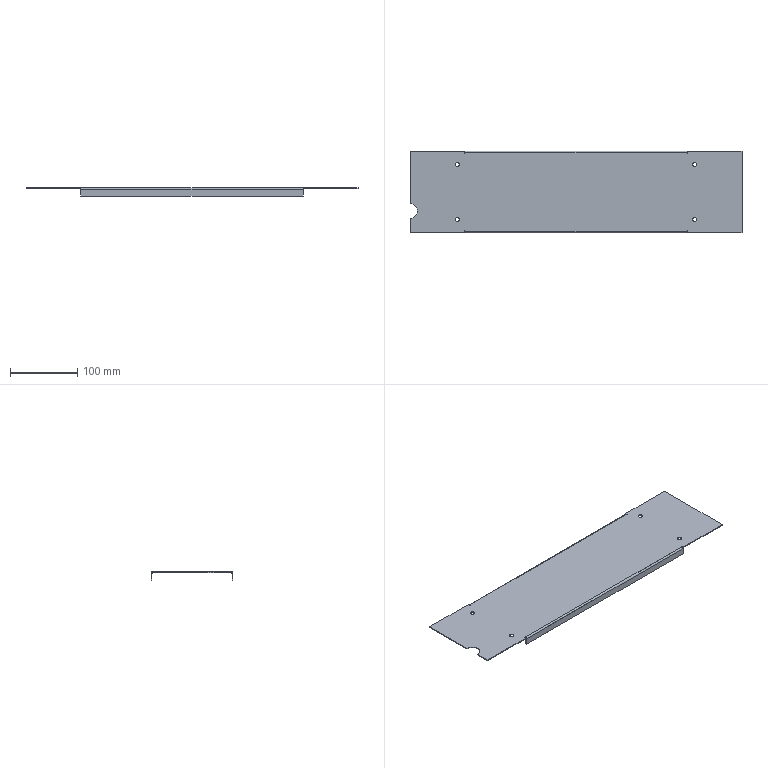Part | SolidWorks | features Cut 2, EdgeFlange 2, FlatPattern 1, SMBaseFlange 1, SheetMetal 1 | 1 solid | 49 faces | box 495 x 122 x 12 mm | volume 80038 mm3 | plane 35 | cylinder 14 | commonest cylinder face diameters 6.5 x8 2.4 x2 4.8 x2 22 x2
STEP:
#1=CARTESIAN_POINT('',(0.,43.5,-1.2));
#2=VERTEX_POINT('',#1);
#3=CARTESIAN_POINT('',(11.,32.5,-1.2));
#4=VERTEX_POINT('',#3);
#5=CARTESIAN_POINT('',(0.,32.5,-1.2));
#6=DIRECTION('',(0.,0.,-1.));
#7=DIRECTION('',(-1.,0.,0.));
#8=AXIS2_PLACEMENT_3D('',#5,#6,#7);
#9=CIRCLE('',#8,11.);
#10=EDGE_CURVE('',#2,#4,#9,.T.);
#11=ORIENTED_EDGE('',*,*,#10,.T.);
#12=CARTESIAN_POINT('',(11.,32.5,0.));
#13=VERTEX_POINT('',#12);
#14=CARTESIAN_POINT('',(11.,32.5,-2.));
#15=DIRECTION('',(0.,0.,1.));
#16=VECTOR('',#15,1000.);
#17=LINE('',#14,#16);
#18=EDGE_CURVE('',#4,#13,#17,.T.);
#19=ORIENTED_EDGE('',*,*,#18,.T.);
#20=CARTESIAN_POINT('',(0.,43.5,0.));
#21=VERTEX_POINT('',#20);
#22=CARTESIAN_POINT('',(0.,32.5,0.));
#23=DIRECTION('',(0.,0.,1.));
#24=DIRECTION('',(1.,0.,0.));
#25=AXIS2_PLACEMENT_3D('',#22,#23,#24);
#26=CIRCLE('',#25,11.);
#27=EDGE_CURVE('',#13,#21,#26,.T.);
#28=ORIENTED_EDGE('',*,*,#27,.T.);
#29=CARTESIAN_POINT('',(0.,43.5,-2.));
#30=DIRECTION('',(0.,0.,-1.));
#31=VECTOR('',#30,1000.);
#32=LINE('',#29,#31);
#33=EDGE_CURVE('',#21,#2,#32,.T.);
#34=ORIENTED_EDGE('',*,*,#33,.T.);
#35=EDGE_LOOP('',(#11,#19,#28,#34));
#36=FACE_OUTER_BOUND('',#35,.T.);
#37=CARTESIAN_POINT('',(0.,32.5,-2.));
#38=DIRECTION('',(0.,0.,1.));
#39=DIRECTION('',(1.,0.,0.));
#40=AXIS2_PLACEMENT_3D('',#37,#38,#39);
#41=CYLINDRICAL_SURFACE('',#40,11.);
#42=ADVANCED_FACE('',(#36),#41,.F.);
#43=CARTESIAN_POINT('',(73.75,20.,-1.2));
#44=VERTEX_POINT('',#43);
#45=CARTESIAN_POINT('',(67.25,20.,-1.2));
#46=VERTEX_POINT('',#45);
#47=CARTESIAN_POINT('',(70.5,20.,-1.2));
#48=DIRECTION('',(0.,0.,-1.));
#49=DIRECTION('',(-1.,0.,0.));
#50=AXIS2_PLACEMENT_3D('',#47,#48,#49);
#51=CIRCLE('',#50,3.25);
#52=EDGE_CURVE('',#44,#46,#51,.T.);
#53=ORIENTED_EDGE('',*,*,#52,.T.);
#54=CARTESIAN_POINT('',(67.25,20.,0.));
#55=VERTEX_POINT('',#54);
#56=CARTESIAN_POINT('',(67.25,20.,-10.));
#57=DIRECTION('',(0.,0.,1.));
#58=VECTOR('',#57,1000.);
#59=LINE('',#56,#58);
#60=EDGE_CURVE('',#46,#55,#59,.T.);
#61=ORIENTED_EDGE('',*,*,#60,.T.);
#62=CARTESIAN_POINT('',(73.75,20.,0.));
#63=VERTEX_POINT('',#62);
#64=CARTESIAN_POINT('',(70.5,20.,0.));
#65=DIRECTION('',(0.,0.,1.));
#66=DIRECTION('',(1.,0.,0.));
#67=AXIS2_PLACEMENT_3D('',#64,#65,#66);
#68=CIRCLE('',#67,3.25);
#69=EDGE_CURVE('',#55,#63,#68,.T.);
#70=ORIENTED_EDGE('',*,*,#69,.T.);
#71=CARTESIAN_POINT('',(73.75,20.,-10.));
#72=DIRECTION('',(0.,0.,1.));
#73=VECTOR('',#72,1000.);
#74=LINE('',#71,#73);
#75=EDGE_CURVE('',#44,#63,#74,.T.);
#76=ORIENTED_EDGE('',*,*,#75,.F.);
#77=EDGE_LOOP('',(#53,#61,#70,#76));
#78=FACE_OUTER_BOUND('',#77,.T.);
#79=CARTESIAN_POINT('',(70.5,20.,-10.));
#80=DIRECTION('',(0.,0.,1.));
#81=DIRECTION('',(1.,0.,0.));
#82=AXIS2_PLACEMENT_3D('',#79,#80,#81);
#83=CYLINDRICAL_SURFACE('',#82,3.25);
#84=ADVANCED_FACE('',(#78),#83,.F.);
#85=CARTESIAN_POINT('',(427.75,20.,-1.2));
#86=VERTEX_POINT('',#85);
#87=CARTESIAN_POINT('',(421.25,20.,-1.2));
#88=VERTEX_POINT('',#87);
#89=CARTESIAN_POINT('',(424.5,20.,-1.2));
#90=DIRECTION('',(0.,0.,-1.));
#91=DIRECTION('',(-1.,0.,0.));
#92=AXIS2_PLACEMENT_3D('',#89,#90,#91);
#93=CIRCLE('',#92,3.25);
#94=EDGE_CURVE('',#86,#88,#93,.T.);
#95=ORIENTED_EDGE('',*,*,#94,.T.);
#96=CARTESIAN_POINT('',(421.25,20.,0.));
#97=VERTEX_POINT('',#96);
#98=CARTESIAN_POINT('',(421.25,20.,-10.));
#99=DIRECTION('',(0.,0.,1.));
#100=VECTOR('',#99,1000.);
#101=LINE('',#98,#100);
#102=EDGE_CURVE('',#88,#97,#101,.T.);
#103=ORIENTED_EDGE('',*,*,#102,.T.);
#104=CARTESIAN_POINT('',(427.75,20.,0.));
#105=VERTEX_POINT('',#104);
#106=CARTESIAN_POINT('',(424.5,20.,0.));
#107=DIRECTION('',(0.,0.,1.));
#108=DIRECTION('',(-1.,0.,0.));
#109=AXIS2_PLACEMENT_3D('',#106,#107,#108);
#110=CIRCLE('',#109,3.25);
#111=EDGE_CURVE('',#97,#105,#110,.T.);
#112=ORIENTED_EDGE('',*,*,#111,.T.);
#113=CARTESIAN_POINT('',(427.75,20.,-10.));
#114=DIRECTION('',(0.,0.,1.));
#115=VECTOR('',#114,1000.);
#116=LINE('',#113,#115);
#117=EDGE_CURVE('',#86,#105,#116,.T.);
#118=ORIENTED_EDGE('',*,*,#117,.F.);
#119=EDGE_LOOP('',(#95,#103,#112,#118));
#120=FACE_OUTER_BOUND('',#119,.T.);
#121=CARTESIAN_POINT('',(424.5,20.,-10.));
#122=DIRECTION('',(0.,0.,1.));
#123=DIRECTION('',(1.,0.,0.));
#124=AXIS2_PLACEMENT_3D('',#121,#122,#123);
#125=CYLINDRICAL_SURFACE('',#124,3.25);
#126=ADVANCED_FACE('',(#120),#125,.F.);
#127=CARTESIAN_POINT('',(427.75,102.,-1.2));
#128=VERTEX_POINT('',#127);
#129=CARTESIAN_POINT('',(421.25,102.,-1.2));
#130=VERTEX_POINT('',#129);
#131=CARTESIAN_POINT('',(424.5,102.,-1.2));
#132=DIRECTION('',(0.,0.,-1.));
#133=DIRECTION('',(-1.,0.,0.));
#134=AXIS2_PLACEMENT_3D('',#131,#132,#133);
#135=CIRCLE('',#134,3.25);
#136=EDGE_CURVE('',#128,#130,#135,.T.);
#137=ORIENTED_EDGE('',*,*,#136,.T.);
#138=CARTESIAN_POINT('',(421.25,102.,0.));
#139=VERTEX_POINT('',#138);
#140=CARTESIAN_POINT('',(421.25,102.,-10.));
#141=DIRECTION('',(0.,0.,1.));
#142=VECTOR('',#141,1000.);
#143=LINE('',#140,#142);
#144=EDGE_CURVE('',#130,#139,#143,.T.);
#145=ORIENTED_EDGE('',*,*,#144,.T.);
#146=CARTESIAN_POINT('',(427.75,102.,0.));
#147=VERTEX_POINT('',#146);
#148=CARTESIAN_POINT('',(424.5,102.,0.));
#149=DIRECTION('',(0.,0.,1.));
#150=DIRECTION('',(-1.,0.,0.));
#151=AXIS2_PLACEMENT_3D('',#148,#149,#150);
#152=CIRCLE('',#151,3.25);
#153=EDGE_CURVE('',#139,#147,#152,.T.);
#154=ORIENTED_EDGE('',*,*,#153,.T.);
#155=CARTESIAN_POINT('',(427.75,102.,-10.));
#156=DIRECTION('',(0.,0.,1.));
#157=VECTOR('',#156,1000.);
#158=LINE('',#155,#157);
#159=EDGE_CURVE('',#128,#147,#158,.T.);
#160=ORIENTED_EDGE('',*,*,#159,.F.);
#161=EDGE_LOOP('',(#137,#145,#154,#160));
#162=FACE_OUTER_BOUND('',#161,.T.);
#163=CARTESIAN_POINT('',(424.5,102.,-10.));
#164=DIRECTION('',(0.,0.,1.));
#165=DIRECTION('',(1.,0.,0.));
#166=AXIS2_PLACEMENT_3D('',#163,#164,#165);
#167=CYLINDRICAL_SURFACE('',#166,3.25);
#168=ADVANCED_FACE('',(#162),#167,.F.);
#169=CARTESIAN_POINT('',(73.75,102.,-1.2));
#170=VERTEX_POINT('',#169);
#171=CARTESIAN_POINT('',(67.25,102.,-1.2));
#172=VERTEX_POINT('',#171);
#173=CARTESIAN_POINT('',(70.5,102.,-1.2));
#174=DIRECTION('',(0.,0.,-1.));
#175=DIRECTION('',(-1.,0.,0.));
#176=AXIS2_PLACEMENT_3D('',#173,#174,#175);
#177=CIRCLE('',#176,3.25);
#178=EDGE_CURVE('',#170,#172,#177,.T.);
#179=ORIENTED_EDGE('',*,*,#178,.T.);
#180=CARTESIAN_POINT('',(67.25,102.,0.));
#181=VERTEX_POINT('',#180);
#182=CARTESIAN_POINT('',(67.25,102.,-10.));
#183=DIRECTION('',(0.,0.,1.));
#184=VECTOR('',#183,1000.);
#185=LINE('',#182,#184);
#186=EDGE_CURVE('',#172,#181,#185,.T.);
#187=ORIENTED_EDGE('',*,*,#186,.T.);
#188=CARTESIAN_POINT('',(73.75,102.,0.));
#189=VERTEX_POINT('',#188);
#190=CARTESIAN_POINT('',(70.5,102.,0.));
#191=DIRECTION('',(0.,0.,1.));
#192=DIRECTION('',(1.,0.,0.));
#193=AXIS2_PLACEMENT_3D('',#190,#191,#192);
#194=CIRCLE('',#193,3.25);
#195=EDGE_CURVE('',#181,#189,#194,.T.);
#196=ORIENTED_EDGE('',*,*,#195,.T.);
#197=CARTESIAN_POINT('',(73.75,102.,-10.));
#198=DIRECTION('',(0.,0.,1.));
#199=VECTOR('',#198,1000.);
#200=LINE('',#197,#199);
#201=EDGE_CURVE('',#170,#189,#200,.T.);
#202=ORIENTED_EDGE('',*,*,#201,.F.);
#203=EDGE_LOOP('',(#179,#187,#196,#202));
#204=FACE_OUTER_BOUND('',#203,.T.);
#205=CARTESIAN_POINT('',(70.5,102.,-10.));
#206=DIRECTION('',(0.,0.,1.));
#207=DIRECTION('',(1.,0.,0.));
#208=AXIS2_PLACEMENT_3D('',#205,#206,#207);
#209=CYLINDRICAL_SURFACE('',#208,3.25);
#210=ADVANCED_FACE('',(#204),#209,.F.);
#211=CARTESIAN_POINT('',(0.,21.5,-1.2));
#212=VERTEX_POINT('',#211);
#213=CARTESIAN_POINT('',(0.,21.5,0.));
#214=VERTEX_POINT('',#213);
#215=CARTESIAN_POINT('',(0.,21.5,-2.));
#216=DIRECTION('',(0.,0.,1.));
#217=VECTOR('',#216,1000.);
#218=LINE('',#215,#217);
#219=EDGE_CURVE('',#212,#214,#218,.T.);
#220=ORIENTED_EDGE('',*,*,#219,.F.);
#221=CARTESIAN_POINT('',(0.,0.,-1.2));
#222=VERTEX_POINT('',#221);
#223=CARTESIAN_POINT('',(0.,0.,-1.2));
#224=DIRECTION('',(0.,-1.,0.));
#225=VECTOR('',#224,1000.);
#226=LINE('',#223,#225);
#227=EDGE_CURVE('',#212,#222,#226,.T.);
#228=ORIENTED_EDGE('',*,*,#227,.T.);
#229=CARTESIAN_POINT('',(0.,0.,0.));
#230=VERTEX_POINT('',#229);
#231=CARTESIAN_POINT('',(0.,0.,-1.2));
#232=DIRECTION('',(0.,0.,1.));
#233=VECTOR('',#232,1000.);
#234=LINE('',#231,#233);
#235=EDGE_CURVE('',#222,#230,#234,.T.);
#236=ORIENTED_EDGE('',*,*,#235,.T.);
#237=CARTESIAN_POINT('',(0.,0.,0.));
#238=DIRECTION('',(0.,-1.,0.));
#239=VECTOR('',#238,1000.);
#240=LINE('',#237,#239);
#241=EDGE_CURVE('',#214,#230,#240,.T.);
#242=ORIENTED_EDGE('',*,*,#241,.F.);
#243=EDGE_LOOP('',(#220,#228,#236,#242));
#244=FACE_OUTER_BOUND('',#243,.T.);
#245=CARTESIAN_POINT('',(0.,0.,-1.2));
#246=DIRECTION('',(-1.,0.,0.));
#247=DIRECTION('',(0.,0.,1.));
#248=AXIS2_PLACEMENT_3D('',#245,#246,#247);
#249=PLANE('',#248);
#250=ADVANCED_FACE('',(#244),#249,.T.);
#251=ORIENTED_EDGE('',*,*,#10,.F.);
#252=CARTESIAN_POINT('',(0.,122.,-1.2));
#253=VERTEX_POINT('',#252);
#254=CARTESIAN_POINT('',(0.,0.,-1.2));
#255=DIRECTION('',(0.,-1.,0.));
#256=VECTOR('',#255,1000.);
#257=LINE('',#254,#256);
#258=EDGE_CURVE('',#253,#2,#257,.T.);
#259=ORIENTED_EDGE('',*,*,#258,.F.);
#260=CARTESIAN_POINT('',(81.4,122.,-1.2));
#261=VERTEX_POINT('',#260);
#262=CARTESIAN_POINT('',(0.,122.,-1.2));
#263=DIRECTION('',(-1.,0.,0.));
#264=VECTOR('',#263,1000.);
#265=LINE('',#262,#264);
#266=EDGE_CURVE('',#261,#253,#265,.T.);
#267=ORIENTED_EDGE('',*,*,#266,.F.);
#268=CARTESIAN_POINT('',(81.4,119.,-1.2));
#269=VERTEX_POINT('',#268);
#270=CARTESIAN_POINT('',(81.4,119.,-1.2));
#271=DIRECTION('',(0.,1.,0.));
#272=VECTOR('',#271,1000.);
#273=LINE('',#270,#272);
#274=EDGE_CURVE('',#269,#261,#273,.T.);
#275=ORIENTED_EDGE('',*,*,#274,.F.);
#276=CARTESIAN_POINT('',(82.,119.,-1.2));
#277=VERTEX_POINT('',#276);
#278=CARTESIAN_POINT('',(82.,119.,-1.2));
#279=DIRECTION('',(-1.,0.,0.));
#280=VECTOR('',#279,1000.);
#281=LINE('',#278,#280);
#282=EDGE_CURVE('',#277,#269,#281,.T.);
#283=ORIENTED_EDGE('',*,*,#282,.F.);
#284=CARTESIAN_POINT('',(82.,119.6,-1.2));
#285=VERTEX_POINT('',#284);
#286=CARTESIAN_POINT('',(82.,119.6,-1.2));
#287=DIRECTION('',(0.,-1.,0.));
#288=VECTOR('',#287,1000.);
#289=LINE('',#286,#288);
#290=EDGE_CURVE('',#285,#277,#289,.T.);
#291=ORIENTED_EDGE('',*,*,#290,.F.);
#292=CARTESIAN_POINT('',(413.,119.6,-1.2));
#293=VERTEX_POINT('',#292);
#294=CARTESIAN_POINT('',(413.,119.6,-1.2));
#295=DIRECTION('',(-1.,0.,0.));
#296=VECTOR('',#295,1000.);
#297=LINE('',#294,#296);
#298=EDGE_CURVE('',#293,#285,#297,.T.);
#299=ORIENTED_EDGE('',*,*,#298,.F.);
#300=CARTESIAN_POINT('',(413.,119.,-1.2));
#301=VERTEX_POINT('',#300);
#302=CARTESIAN_POINT('',(413.,119.,-1.2));
#303=DIRECTION('',(0.,1.,0.));
#304=VECTOR('',#303,1000.);
#305=LINE('',#302,#304);
#306=EDGE_CURVE('',#301,#293,#305,.T.);
#307=ORIENTED_EDGE('',*,*,#306,.F.);
#308=CARTESIAN_POINT('',(413.6,119.,-1.2));
#309=VERTEX_POINT('',#308);
#310=CARTESIAN_POINT('',(413.6,119.,-1.2));
#311=DIRECTION('',(-1.,0.,0.));
#312=VECTOR('',#311,1000.);
#313=LINE('',#310,#312);
#314=EDGE_CURVE('',#309,#301,#313,.T.);
#315=ORIENTED_EDGE('',*,*,#314,.F.);
#316=CARTESIAN_POINT('',(413.6,122.,-1.2));
#317=VERTEX_POINT('',#316);
#318=CARTESIAN_POINT('',(413.6,122.,-1.2));
#319=DIRECTION('',(0.,-1.,0.));
#320=VECTOR('',#319,1000.);
#321=LINE('',#318,#320);
#322=EDGE_CURVE('',#317,#309,#321,.T.);
#323=ORIENTED_EDGE('',*,*,#322,.F.);
#324=CARTESIAN_POINT('',(495.,122.,-1.2));
#325=VERTEX_POINT('',#324);
#326=CARTESIAN_POINT('',(0.,122.,-1.2));
#327=DIRECTION('',(-1.,0.,0.));
#328=VECTOR('',#327,1000.);
#329=LINE('',#326,#328);
#330=EDGE_CURVE('',#325,#317,#329,.T.);
#331=ORIENTED_EDGE('',*,*,#330,.F.);
#332=CARTESIAN_POINT('',(495.,0.,-1.2));
#333=VERTEX_POINT('',#332);
#334=CARTESIAN_POINT('',(495.,0.,-1.2));
#335=DIRECTION('',(0.,1.,0.));
#336=VECTOR('',#335,1000.);
#337=LINE('',#334,#336);
#338=EDGE_CURVE('',#333,#325,#337,.T.);
#339=ORIENTED_EDGE('',*,*,#338,.F.);
#340=CARTESIAN_POINT('',(413.6,0.,-1.2));
#341=VERTEX_POINT('',#340);
#342=CARTESIAN_POINT('',(0.,0.,-1.2));
#343=DIRECTION('',(1.,0.,0.));
#344=VECTOR('',#343,1000.);
#345=LINE('',#342,#344);
#346=EDGE_CURVE('',#341,#333,#345,.T.);
#347=ORIENTED_EDGE('',*,*,#346,.F.);
#348=CARTESIAN_POINT('',(413.6,3.,-1.2));
#349=VERTEX_POINT('',#348);
#350=CARTESIAN_POINT('',(413.6,3.,-1.2));
#351=DIRECTION('',(0.,-1.,0.));
#352=VECTOR('',#351,1000.);
#353=LINE('',#350,#352);
#354=EDGE_CURVE('',#349,#341,#353,.T.);
#355=ORIENTED_EDGE('',*,*,#354,.F.);
#356=CARTESIAN_POINT('',(413.,3.,-1.2));
#357=VERTEX_POINT('',#356);
#358=CARTESIAN_POINT('',(413.,3.,-1.2));
#359=DIRECTION('',(1.,0.,0.));
#360=VECTOR('',#359,1000.);
#361=LINE('',#358,#360);
#362=EDGE_CURVE('',#357,#349,#361,.T.);
#363=ORIENTED_EDGE('',*,*,#362,.F.);
#364=CARTESIAN_POINT('',(413.,2.4,-1.2));
#365=VERTEX_POINT('',#364);
#366=CARTESIAN_POINT('',(413.,2.4,-1.2));
#367=DIRECTION('',(0.,1.,0.));
#368=VECTOR('',#367,1000.);
#369=LINE('',#366,#368);
#370=EDGE_CURVE('',#365,#357,#369,.T.);
#371=ORIENTED_EDGE('',*,*,#370,.F.);
#372=CARTESIAN_POINT('',(82.,2.4,-1.2));
#373=VERTEX_POINT('',#372);
#374=CARTESIAN_POINT('',(82.,2.4,-1.2));
#375=DIRECTION('',(1.,0.,0.));
#376=VECTOR('',#375,1000.);
#377=LINE('',#374,#376);
#378=EDGE_CURVE('',#373,#365,#377,.T.);
#379=ORIENTED_EDGE('',*,*,#378,.F.);
#380=CARTESIAN_POINT('',(82.,3.,-1.2));
#381=VERTEX_POINT('',#380);
#382=CARTESIAN_POINT('',(82.,3.,-1.2));
#383=DIRECTION('',(0.,-1.,0.));
#384=VECTOR('',#383,1000.);
#385=LINE('',#382,#384);
#386=EDGE_CURVE('',#381,#373,#385,.T.);
#387=ORIENTED_EDGE('',*,*,#386,.F.);
#388=CARTESIAN_POINT('',(81.4,3.,-1.2));
#389=VERTEX_POINT('',#388);
#390=CARTESIAN_POINT('',(81.4,3.,-1.2));
#391=DIRECTION('',(1.,0.,0.));
#392=VECTOR('',#391,1000.);
#393=LINE('',#390,#392);
#394=EDGE_CURVE('',#389,#381,#393,.T.);
#395=ORIENTED_EDGE('',*,*,#394,.F.);
#396=CARTESIAN_POINT('',(81.4,0.,-1.2));
#397=VERTEX_POINT('',#396);
#398=CARTESIAN_POINT('',(81.4,0.,-1.2));
#399=DIRECTION('',(0.,1.,0.));
#400=VECTOR('',#399,1000.);
#401=LINE('',#398,#400);
#402=EDGE_CURVE('',#397,#389,#401,.T.);
#403=ORIENTED_EDGE('',*,*,#402,.F.);
#404=CARTESIAN_POINT('',(0.,0.,-1.2));
#405=DIRECTION('',(1.,0.,0.));
#406=VECTOR('',#405,1000.);
#407=LINE('',#404,#406);
#408=EDGE_CURVE('',#222,#397,#407,.T.);
#409=ORIENTED_EDGE('',*,*,#408,.F.);
#410=ORIENTED_EDGE('',*,*,#227,.F.);
#411=CARTESIAN_POINT('',(0.,32.5,-1.2));
#412=DIRECTION('',(0.,0.,-1.));
#413=DIRECTION('',(-1.,0.,0.));
#414=AXIS2_PLACEMENT_3D('',#411,#412,#413);
#415=CIRCLE('',#414,11.);
#416=EDGE_CURVE('',#4,#212,#415,.T.);
#417=ORIENTED_EDGE('',*,*,#416,.F.);
#418=EDGE_LOOP('',(#251,#259,#267,#275,#283,#291,#299,#307,#315,#323,#331,#339,#347,#355,#363,#371,#379,#387,#395,#403,#409,#410,#417));
#419=FACE_OUTER_BOUND('',#418,.T.);
#420=ORIENTED_EDGE('',*,*,#52,.F.);
#421=CARTESIAN_POINT('',(70.5,20.,-1.2));
#422=DIRECTION('',(0.,0.,-1.));
#423=DIRECTION('',(-1.,0.,0.));
#424=AXIS2_PLACEMENT_3D('',#421,#422,#423);
#425=CIRCLE('',#424,3.25);
#426=EDGE_CURVE('',#46,#44,#425,.T.);
#427=ORIENTED_EDGE('',*,*,#426,.F.);
#428=EDGE_LOOP('',(#420,#427));
#429=FACE_BOUND('',#428,.T.);
#430=ORIENTED_EDGE('',*,*,#94,.F.);
#431=CARTESIAN_POINT('',(424.5,20.,-1.2));
#432=DIRECTION('',(0.,0.,-1.));
#433=DIRECTION('',(-1.,0.,0.));
#434=AXIS2_PLACEMENT_3D('',#431,#432,#433);
#435=CIRCLE('',#434,3.25);
#436=EDGE_CURVE('',#88,#86,#435,.T.);
#437=ORIENTED_EDGE('',*,*,#436,.F.);
#438=EDGE_LOOP('',(#430,#437));
#439=FACE_BOUND('',#438,.T.);
#440=ORIENTED_EDGE('',*,*,#136,.F.);
#441=CARTESIAN_POINT('',(424.5,102.,-1.2));
#442=DIRECTION('',(0.,0.,-1.));
#443=DIRECTION('',(-1.,0.,0.));
#444=AXIS2_PLACEMENT_3D('',#441,#442,#443);
#445=CIRCLE('',#444,3.25);
#446=EDGE_CURVE('',#130,#128,#445,.T.);
#447=ORIENTED_EDGE('',*,*,#446,.F.);
#448=EDGE_LOOP('',(#440,#447));
#449=FACE_BOUND('',#448,.T.);
#450=ORIENTED_EDGE('',*,*,#178,.F.);
#451=CARTESIAN_POINT('',(70.5,102.,-1.2));
#452=DIRECTION('',(0.,0.,-1.));
#453=DIRECTION('',(-1.,0.,0.));
#454=AXIS2_PLACEMENT_3D('',#451,#452,#453);
#455=CIRCLE('',#454,3.25);
#456=EDGE_CURVE('',#172,#170,#455,.T.);
#457=ORIENTED_EDGE('',*,*,#456,.F.);
#458=EDGE_LOOP('',(#450,#457));
#459=FACE_BOUND('',#458,.T.);
#460=CARTESIAN_POINT('',(0.,0.,-1.2));
#461=DIRECTION('',(0.,0.,-1.));
#462=DIRECTION('',(-1.,0.,0.));
#463=AXIS2_PLACEMENT_3D('',#460,#461,#462);
#464=PLANE('',#463);
#465=ADVANCED_FACE('',(#419,#429,#439,#449,#459),#464,.T.);
#466=CARTESIAN_POINT('',(70.5,20.,0.));
#467=DIRECTION('',(0.,0.,1.));
#468=DIRECTION('',(1.,0.,0.));
#469=AXIS2_PLACEMENT_3D('',#466,#467,#468);
#470=CIRCLE('',#469,3.25);
#471=EDGE_CURVE('',#63,#55,#470,.T.);
#472=ORIENTED_EDGE('',*,*,#471,.F.);
#473=ORIENTED_EDGE('',*,*,#69,.F.);
#474=EDGE_LOOP('',(#472,#473));
#475=FACE_BOUND('',#474,.T.);
#476=CARTESIAN_POINT('',(424.5,20.,0.));
#477=DIRECTION('',(0.,0.,1.));
#478=DIRECTION('',(-1.,0.,0.));
#479=AXIS2_PLACEMENT_3D('',#476,#477,#478);
#480=CIRCLE('',#479,3.25);
#481=EDGE_CURVE('',#105,#97,#480,.T.);
#482=ORIENTED_EDGE('',*,*,#481,.F.);
#483=ORIENTED_EDGE('',*,*,#111,.F.);
#484=EDGE_LOOP('',(#482,#483));
#485=FACE_BOUND('',#484,.T.);
#486=CARTESIAN_POINT('',(424.5,102.,0.));
#487=DIRECTION('',(0.,0.,1.));
#488=DIRECTION('',(-1.,0.,0.));
#489=AXIS2_PLACEMENT_3D('',#486,#487,#488);
#490=CIRCLE('',#489,3.25);
#491=EDGE_CURVE('',#147,#139,#490,.T.);
#492=ORIENTED_EDGE('',*,*,#491,.F.);
#493=ORIENTED_EDGE('',*,*,#153,.F.);
#494=EDGE_LOOP('',(#492,#493));
#495=FACE_BOUND('',#494,.T.);
#496=CARTESIAN_POINT('',(70.5,102.,0.));
#497=DIRECTION('',(0.,0.,1.));
#498=DIRECTION('',(1.,0.,0.));
#499=AXIS2_PLACEMENT_3D('',#496,#497,#498);
#500=CIRCLE('',#499,3.25);
#501=EDGE_CURVE('',#189,#181,#500,.T.);
#502=ORIENTED_EDGE('',*,*,#501,.F.);
#503=ORIENTED_EDGE('',*,*,#195,.F.);
#504=EDGE_LOOP('',(#502,#503));
#505=FACE_BOUND('',#504,.T.);
#506=CARTESIAN_POINT('',(0.,122.,0.));
#507=VERTEX_POINT('',#506);
#508=CARTESIAN_POINT('',(0.,0.,0.));
#509=DIRECTION('',(0.,-1.,0.));
#510=VECTOR('',#509,1000.);
#511=LINE('',#508,#510);
#512=EDGE_CURVE('',#507,#21,#511,.T.);
#513=ORIENTED_EDGE('',*,*,#512,.T.);
#514=ORIENTED_EDGE('',*,*,#27,.F.);
#515=CARTESIAN_POINT('',(0.,32.5,0.));
#516=DIRECTION('',(0.,0.,1.));
#517=DIRECTION('',(1.,0.,0.));
#518=AXIS2_PLACEMENT_3D('',#515,#516,#517);
#519=CIRCLE('',#518,11.);
#520=EDGE_CURVE('',#214,#13,#519,.T.);
#521=ORIENTED_EDGE('',*,*,#520,.F.);
#522=ORIENTED_EDGE('',*,*,#241,.T.);
#523=CARTESIAN_POINT('',(81.4,0.,0.));
#524=VERTEX_POINT('',#523);
#525=CARTESIAN_POINT('',(0.,0.,0.));
#526=DIRECTION('',(1.,0.,0.));
#527=VECTOR('',#526,1000.);
#528=LINE('',#525,#527);
#529=EDGE_CURVE('',#230,#524,#528,.T.);
#530=ORIENTED_EDGE('',*,*,#529,.T.);
#531=CARTESIAN_POINT('',(81.4,3.,0.));
#532=VERTEX_POINT('',#531);
#533=CARTESIAN_POINT('',(81.4,0.,0.));
#534=DIRECTION('',(0.,-1.,0.));
#535=VECTOR('',#534,1000.);
#536=LINE('',#533,#535);
#537=EDGE_CURVE('',#532,#524,#536,.T.);
#538=ORIENTED_EDGE('',*,*,#537,.F.);
#539=CARTESIAN_POINT('',(82.,3.,0.));
#540=VERTEX_POINT('',#539);
#541=CARTESIAN_POINT('',(0.,3.,0.));
#542=DIRECTION('',(-1.,0.,0.));
#543=VECTOR('',#542,1000.);
#544=LINE('',#541,#543);
#545=EDGE_CURVE('',#540,#532,#544,.T.);
#546=ORIENTED_EDGE('',*,*,#545,.F.);
#547=CARTESIAN_POINT('',(82.,2.4,0.));
#548=VERTEX_POINT('',#547);
#549=CARTESIAN_POINT('',(82.,0.,0.));
#550=DIRECTION('',(0.,1.,0.));
#551=VECTOR('',#550,1000.);
#552=LINE('',#549,#551);
#553=EDGE_CURVE('',#548,#540,#552,.T.);
#554=ORIENTED_EDGE('',*,*,#553,.F.);
#555=CARTESIAN_POINT('',(413.,2.4,0.));
#556=VERTEX_POINT('',#555);
#557=CARTESIAN_POINT('',(82.,2.4,0.));
#558=DIRECTION('',(1.,0.,0.));
#559=VECTOR('',#558,1000.);
#560=LINE('',#557,#559);
#561=EDGE_CURVE('',#548,#556,#560,.T.);
#562=ORIENTED_EDGE('',*,*,#561,.T.);
#563=CARTESIAN_POINT('',(413.,3.,0.));
#564=VERTEX_POINT('',#563);
#565=CARTESIAN_POINT('',(413.,0.,0.));
#566=DIRECTION('',(0.,-1.,0.));
#567=VECTOR('',#566,1000.);
#568=LINE('',#565,#567);
#569=EDGE_CURVE('',#564,#556,#568,.T.);
#570=ORIENTED_EDGE('',*,*,#569,.F.);
#571=CARTESIAN_POINT('',(413.6,3.,0.));
#572=VERTEX_POINT('',#571);
#573=CARTESIAN_POINT('',(0.,3.,0.));
#574=DIRECTION('',(-1.,0.,0.));
#575=VECTOR('',#574,1000.);
#576=LINE('',#573,#575);
#577=EDGE_CURVE('',#572,#564,#576,.T.);
#578=ORIENTED_EDGE('',*,*,#577,.F.);
#579=CARTESIAN_POINT('',(413.6,0.,0.));
#580=VERTEX_POINT('',#579);
#581=CARTESIAN_POINT('',(413.6,0.,0.));
#582=DIRECTION('',(0.,1.,0.));
#583=VECTOR('',#582,1000.);
#584=LINE('',#581,#583);
#585=EDGE_CURVE('',#580,#572,#584,.T.);
#586=ORIENTED_EDGE('',*,*,#585,.F.);
#587=CARTESIAN_POINT('',(495.,0.,0.));
#588=VERTEX_POINT('',#587);
#589=CARTESIAN_POINT('',(0.,0.,0.));
#590=DIRECTION('',(1.,0.,0.));
#591=VECTOR('',#590,1000.);
#592=LINE('',#589,#591);
#593=EDGE_CURVE('',#580,#588,#592,.T.);
#594=ORIENTED_EDGE('',*,*,#593,.T.);
#595=CARTESIAN_POINT('',(495.,122.,0.));
#596=VERTEX_POINT('',#595);
#597=CARTESIAN_POINT('',(495.,0.,0.));
#598=DIRECTION('',(0.,1.,0.));
#599=VECTOR('',#598,1000.);
#600=LINE('',#597,#599);
#601=EDGE_CURVE('',#588,#596,#600,.T.);
#602=ORIENTED_EDGE('',*,*,#601,.T.);
#603=CARTESIAN_POINT('',(413.6,122.,0.));
#604=VERTEX_POINT('',#603);
#605=CARTESIAN_POINT('',(0.,122.,0.));
#606=DIRECTION('',(-1.,0.,0.));
#607=VECTOR('',#606,1000.);
#608=LINE('',#605,#607);
#609=EDGE_CURVE('',#596,#604,#608,.T.);
#610=ORIENTED_EDGE('',*,*,#609,.T.);
#611=CARTESIAN_POINT('',(413.6,119.,0.));
#612=VERTEX_POINT('',#611);
#613=CARTESIAN_POINT('',(413.6,0.,0.));
#614=DIRECTION('',(0.,1.,0.));
#615=VECTOR('',#614,1000.);
#616=LINE('',#613,#615);
#617=EDGE_CURVE('',#612,#604,#616,.T.);
#618=ORIENTED_EDGE('',*,*,#617,.F.);
#619=CARTESIAN_POINT('',(413.,119.,0.));
#620=VERTEX_POINT('',#619);
#621=CARTESIAN_POINT('',(0.,119.,0.));
#622=DIRECTION('',(1.,0.,0.));
#623=VECTOR('',#622,1000.);
#624=LINE('',#621,#623);
#625=EDGE_CURVE('',#620,#612,#624,.T.);
#626=ORIENTED_EDGE('',*,*,#625,.F.);
#627=CARTESIAN_POINT('',(413.,119.6,0.));
#628=VERTEX_POINT('',#627);
#629=CARTESIAN_POINT('',(413.,0.,0.));
#630=DIRECTION('',(0.,-1.,0.));
#631=VECTOR('',#630,1000.);
#632=LINE('',#629,#631);
#633=EDGE_CURVE('',#628,#620,#632,.T.);
#634=ORIENTED_EDGE('',*,*,#633,.F.);
#635=CARTESIAN_POINT('',(82.,119.6,0.));
#636=VERTEX_POINT('',#635);
#637=CARTESIAN_POINT('',(413.,119.6,0.));
#638=DIRECTION('',(-1.,0.,0.));
#639=VECTOR('',#638,1000.);
#640=LINE('',#637,#639);
#641=EDGE_CURVE('',#628,#636,#640,.T.);
#642=ORIENTED_EDGE('',*,*,#641,.T.);
#643=CARTESIAN_POINT('',(82.,119.,0.));
#644=VERTEX_POINT('',#643);
#645=CARTESIAN_POINT('',(82.,0.,0.));
#646=DIRECTION('',(0.,1.,0.));
#647=VECTOR('',#646,1000.);
#648=LINE('',#645,#647);
#649=EDGE_CURVE('',#644,#636,#648,.T.);
#650=ORIENTED_EDGE('',*,*,#649,.F.);
#651=CARTESIAN_POINT('',(81.4,119.,0.));
#652=VERTEX_POINT('',#651);
#653=CARTESIAN_POINT('',(0.,119.,0.));
#654=DIRECTION('',(1.,0.,0.));
#655=VECTOR('',#654,1000.);
#656=LINE('',#653,#655);
#657=EDGE_CURVE('',#652,#644,#656,.T.);
#658=ORIENTED_EDGE('',*,*,#657,.F.);
#659=CARTESIAN_POINT('',(81.4,122.,0.));
#660=VERTEX_POINT('',#659);
#661=CARTESIAN_POINT('',(81.4,0.,0.));
#662=DIRECTION('',(0.,-1.,0.));
#663=VECTOR('',#662,1000.);
#664=LINE('',#661,#663);
#665=EDGE_CURVE('',#660,#652,#664,.T.);
#666=ORIENTED_EDGE('',*,*,#665,.F.);
#667=CARTESIAN_POINT('',(0.,122.,0.));
#668=DIRECTION('',(-1.,0.,0.));
#669=VECTOR('',#668,1000.);
#670=LINE('',#667,#669);
#671=EDGE_CURVE('',#660,#507,#670,.T.);
#672=ORIENTED_EDGE('',*,*,#671,.T.);
#673=EDGE_LOOP('',(#513,#514,#521,#522,#530,#538,#546,#554,#562,#570,#578,#586,#594,#602,#610,#618,#626,#634,#642,#650,#658,#666,#672));
#674=FACE_OUTER_BOUND('',#673,.T.);
#675=CARTESIAN_POINT('',(0.,0.,0.));
#676=DIRECTION('',(0.,0.,-1.));
#677=DIRECTION('',(-1.,0.,0.));
#678=AXIS2_PLACEMENT_3D('',#675,#676,#677);
#679=PLANE('',#678);
#680=ADVANCED_FACE('',(#475,#485,#495,#505,#674),#679,.F.);
#681=ORIENTED_EDGE('',*,*,#330,.T.);
#682=CARTESIAN_POINT('',(413.6,122.,-1.2));
#683=DIRECTION('',(0.,0.,1.));
#684=VECTOR('',#683,1000.);
#685=LINE('',#682,#684);
#686=EDGE_CURVE('',#317,#604,#685,.T.);
#687=ORIENTED_EDGE('',*,*,#686,.T.);
#688=ORIENTED_EDGE('',*,*,#609,.F.);
#689=CARTESIAN_POINT('',(495.,122.,-1.2));
#690=DIRECTION('',(0.,0.,1.));
#691=VECTOR('',#690,1000.);
#692=LINE('',#689,#691);
#693=EDGE_CURVE('',#325,#596,#692,.T.);
#694=ORIENTED_EDGE('',*,*,#693,.F.);
#695=EDGE_LOOP('',(#681,#687,#688,#694));
#696=FACE_OUTER_BOUND('',#695,.T.);
#697=CARTESIAN_POINT('',(0.,122.,-1.2));
#698=DIRECTION('',(0.,1.,0.));
#699=DIRECTION('',(0.,0.,1.));
#700=AXIS2_PLACEMENT_3D('',#697,#698,#699);
#701=PLANE('',#700);
#702=ADVANCED_FACE('',(#696),#701,.T.);
#703=ORIENTED_EDGE('',*,*,#671,.F.);
#704=CARTESIAN_POINT('',(81.4,122.,-1.2));
#705=DIRECTION('',(0.,0.,1.));
#706=VECTOR('',#705,1000.);
#707=LINE('',#704,#706);
#708=EDGE_CURVE('',#261,#660,#707,.T.);
#709=ORIENTED_EDGE('',*,*,#708,.F.);
#710=ORIENTED_EDGE('',*,*,#266,.T.);
#711=CARTESIAN_POINT('',(0.,122.,-1.2));
#712=DIRECTION('',(0.,0.,1.));
#713=VECTOR('',#712,1000.);
#714=LINE('',#711,#713);
#715=EDGE_CURVE('',#253,#507,#714,.T.);
#716=ORIENTED_EDGE('',*,*,#715,.T.);
#717=EDGE_LOOP('',(#703,#709,#710,#716));
#718=FACE_OUTER_BOUND('',#717,.T.);
#719=CARTESIAN_POINT('',(0.,122.,-1.2));
#720=DIRECTION('',(0.,1.,0.));
#721=DIRECTION('',(0.,0.,1.));
#722=AXIS2_PLACEMENT_3D('',#719,#720,#721);
#723=PLANE('',#722);
#724=ADVANCED_FACE('',(#718),#723,.T.);
#725=ORIENTED_EDGE('',*,*,#408,.T.);
#726=CARTESIAN_POINT('',(81.4,0.,-1.2));
#727=DIRECTION('',(0.,0.,1.));
#728=VECTOR('',#727,1000.);
#729=LINE('',#726,#728);
#730=EDGE_CURVE('',#397,#524,#729,.T.);
#731=ORIENTED_EDGE('',*,*,#730,.T.);
#732=ORIENTED_EDGE('',*,*,#529,.F.);
#733=ORIENTED_EDGE('',*,*,#235,.F.);
#734=EDGE_LOOP('',(#725,#731,#732,#733));
#735=FACE_OUTER_BOUND('',#734,.T.);
#736=CARTESIAN_POINT('',(0.,0.,-1.2));
#737=DIRECTION('',(0.,-1.,0.));
#738=DIRECTION('',(0.,0.,-1.));
#739=AXIS2_PLACEMENT_3D('',#736,#737,#738);
#740=PLANE('',#739);
#741=ADVANCED_FACE('',(#735),#740,.T.);
#742=ORIENTED_EDGE('',*,*,#593,.F.);
#743=CARTESIAN_POINT('',(413.6,0.,-1.2));
#744=DIRECTION('',(0.,0.,1.));
#745=VECTOR('',#744,1000.);
#746=LINE('',#743,#745);
#747=EDGE_CURVE('',#341,#580,#746,.T.);
#748=ORIENTED_EDGE('',*,*,#747,.F.);
#749=ORIENTED_EDGE('',*,*,#346,.T.);
#750=CARTESIAN_POINT('',(495.,0.,-1.2));
#751=DIRECTION('',(0.,0.,1.));
#752=VECTOR('',#751,1000.);
#753=LINE('',#750,#752);
#754=EDGE_CURVE('',#333,#588,#753,.T.);
#755=ORIENTED_EDGE('',*,*,#754,.T.);
#756=EDGE_LOOP('',(#742,#748,#749,#755));
#757=FACE_OUTER_BOUND('',#756,.T.);
#758=CARTESIAN_POINT('',(0.,0.,-1.2));
#759=DIRECTION('',(0.,-1.,0.));
#760=DIRECTION('',(0.,0.,-1.));
#761=AXIS2_PLACEMENT_3D('',#758,#759,#760);
#762=PLANE('',#761);
#763=ADVANCED_FACE('',(#757),#762,.T.);
#764=ORIENTED_EDGE('',*,*,#33,.F.);
#765=ORIENTED_EDGE('',*,*,#512,.F.);
#766=ORIENTED_EDGE('',*,*,#715,.F.);
#767=ORIENTED_EDGE('',*,*,#258,.T.);
#768=EDGE_LOOP('',(#764,#765,#766,#767));
#769=FACE_OUTER_BOUND('',#768,.T.);
#770=CARTESIAN_POINT('',(0.,0.,-1.2));
#771=DIRECTION('',(-1.,0.,0.));
#772=DIRECTION('',(0.,0.,1.));
#773=AXIS2_PLACEMENT_3D('',#770,#771,#772);
#774=PLANE('',#773);
#775=ADVANCED_FACE('',(#769),#774,.T.);
#776=ORIENTED_EDGE('',*,*,#601,.F.);
#777=ORIENTED_EDGE('',*,*,#754,.F.);
#778=ORIENTED_EDGE('',*,*,#338,.T.);
#779=ORIENTED_EDGE('',*,*,#693,.T.);
#780=EDGE_LOOP('',(#776,#777,#778,#779));
#781=FACE_OUTER_BOUND('',#780,.T.);
#782=CARTESIAN_POINT('',(495.,0.,-1.2));
#783=DIRECTION('',(1.,0.,0.));
#784=DIRECTION('',(0.,0.,-1.));
#785=AXIS2_PLACEMENT_3D('',#782,#783,#784);
#786=PLANE('',#785);
#787=ADVANCED_FACE('',(#781),#786,.T.);
#788=CARTESIAN_POINT('',(81.4,3.,-1.2));
#789=DIRECTION('',(0.,0.,1.));
#790=VECTOR('',#789,1000.);
#791=LINE('',#788,#790);
#792=EDGE_CURVE('',#389,#532,#791,.T.);
#793=ORIENTED_EDGE('',*,*,#792,.T.);
#794=ORIENTED_EDGE('',*,*,#537,.T.);
#795=ORIENTED_EDGE('',*,*,#730,.F.);
#796=ORIENTED_EDGE('',*,*,#402,.T.);
#797=EDGE_LOOP('',(#793,#794,#795,#796));
#798=FACE_OUTER_BOUND('',#797,.T.);
#799=CARTESIAN_POINT('',(81.4,0.,-1.2));
#800=DIRECTION('',(1.,0.,0.));
#801=DIRECTION('',(0.,0.,-1.));
#802=AXIS2_PLACEMENT_3D('',#799,#800,#801);
#803=PLANE('',#802);
#804=ADVANCED_FACE('',(#798),#803,.T.);
#805=CARTESIAN_POINT('',(82.,3.,-1.2));
#806=DIRECTION('',(0.,0.,1.));
#807=VECTOR('',#806,1000.);
#808=LINE('',#805,#807);
#809=EDGE_CURVE('',#381,#540,#808,.T.);
#810=ORIENTED_EDGE('',*,*,#809,.T.);
#811=ORIENTED_EDGE('',*,*,#545,.T.);
#812=ORIENTED_EDGE('',*,*,#792,.F.);
#813=ORIENTED_EDGE('',*,*,#394,.T.);
#814=EDGE_LOOP('',(#810,#811,#812,#813));
#815=FACE_OUTER_BOUND('',#814,.T.);
#816=CARTESIAN_POINT('',(81.4,3.,-1.2));
#817=DIRECTION('',(0.,-1.,0.));
#818=DIRECTION('',(0.,0.,-1.));
#819=AXIS2_PLACEMENT_3D('',#816,#817,#818);
#820=PLANE('',#819);
#821=ADVANCED_FACE('',(#815),#820,.T.);
#822=CARTESIAN_POINT('',(82.,2.4,-1.2));
#823=DIRECTION('',(0.,0.,1.));
#824=VECTOR('',#823,1000.);
#825=LINE('',#822,#824);
#826=EDGE_CURVE('',#373,#548,#825,.T.);
#827=ORIENTED_EDGE('',*,*,#826,.T.);
#828=ORIENTED_EDGE('',*,*,#553,.T.);
#829=ORIENTED_EDGE('',*,*,#809,.F.);
#830=ORIENTED_EDGE('',*,*,#386,.T.);
#831=EDGE_LOOP('',(#827,#828,#829,#830));
#832=FACE_OUTER_BOUND('',#831,.T.);
#833=CARTESIAN_POINT('',(82.,3.,-1.2));
#834=DIRECTION('',(-1.,0.,0.));
#835=DIRECTION('',(0.,0.,1.));
#836=AXIS2_PLACEMENT_3D('',#833,#834,#835);
#837=PLANE('',#836);
#838=ADVANCED_FACE('',(#832),#837,.T.);
#839=CARTESIAN_POINT('',(413.,3.,-1.2));
#840=DIRECTION('',(0.,0.,1.));
#841=VECTOR('',#840,1000.);
#842=LINE('',#839,#841);
#843=EDGE_CURVE('',#357,#564,#842,.T.);
#844=ORIENTED_EDGE('',*,*,#843,.T.);
#845=ORIENTED_EDGE('',*,*,#569,.T.);
#846=CARTESIAN_POINT('',(413.,2.4,-1.2));
#847=DIRECTION('',(0.,0.,1.));
#848=VECTOR('',#847,1000.);
#849=LINE('',#846,#848);
#850=EDGE_CURVE('',#365,#556,#849,.T.);
#851=ORIENTED_EDGE('',*,*,#850,.F.);
#852=ORIENTED_EDGE('',*,*,#370,.T.);
#853=EDGE_LOOP('',(#844,#845,#851,#852));
#854=FACE_OUTER_BOUND('',#853,.T.);
#855=CARTESIAN_POINT('',(413.,2.4,-1.2));
#856=DIRECTION('',(1.,0.,0.));
#857=DIRECTION('',(0.,0.,-1.));
#858=AXIS2_PLACEMENT_3D('',#855,#856,#857);
#859=PLANE('',#858);
#860=ADVANCED_FACE('',(#854),#859,.T.);
#861=CARTESIAN_POINT('',(413.6,3.,-1.2));
#862=DIRECTION('',(0.,0.,1.));
#863=VECTOR('',#862,1000.);
#864=LINE('',#861,#863);
#865=EDGE_CURVE('',#349,#572,#864,.T.);
#866=ORIENTED_EDGE('',*,*,#865,.T.);
#867=ORIENTED_EDGE('',*,*,#577,.T.);
#868=ORIENTED_EDGE('',*,*,#843,.F.);
#869=ORIENTED_EDGE('',*,*,#362,.T.);
#870=EDGE_LOOP('',(#866,#867,#868,#869));
#871=FACE_OUTER_BOUND('',#870,.T.);
#872=CARTESIAN_POINT('',(413.,3.,-1.2));
#873=DIRECTION('',(0.,-1.,0.));
#874=DIRECTION('',(0.,0.,-1.));
#875=AXIS2_PLACEMENT_3D('',#872,#873,#874);
#876=PLANE('',#875);
#877=ADVANCED_FACE('',(#871),#876,.T.);
#878=ORIENTED_EDGE('',*,*,#747,.T.);
#879=ORIENTED_EDGE('',*,*,#585,.T.);
#880=ORIENTED_EDGE('',*,*,#865,.F.);
#881=ORIENTED_EDGE('',*,*,#354,.T.);
#882=EDGE_LOOP('',(#878,#879,#880,#881));
#883=FACE_OUTER_BOUND('',#882,.T.);
#884=CARTESIAN_POINT('',(413.6,3.,-1.2));
#885=DIRECTION('',(-1.,0.,0.));
#886=DIRECTION('',(0.,0.,1.));
#887=AXIS2_PLACEMENT_3D('',#884,#885,#886);
#888=PLANE('',#887);
#889=ADVANCED_FACE('',(#883),#888,.T.);
#890=CARTESIAN_POINT('',(413.,1.2,-2.4));
#891=VERTEX_POINT('',#890);
#892=CARTESIAN_POINT('',(413.,0.,-2.4));
#893=VERTEX_POINT('',#892);
#894=CARTESIAN_POINT('',(413.,0.,-2.4));
#895=DIRECTION('',(0.,-1.,0.));
#896=VECTOR('',#895,1000.);
#897=LINE('',#894,#896);
#898=EDGE_CURVE('',#891,#893,#897,.T.);
#899=ORIENTED_EDGE('',*,*,#898,.F.);
#900=CARTESIAN_POINT('',(413.,2.4,-2.4));
#901=DIRECTION('',(1.,0.,0.));
#902=DIRECTION('',(0.,0.,1.));
#903=AXIS2_PLACEMENT_3D('',#900,#901,#902);
#904=CIRCLE('',#903,1.2);
#905=EDGE_CURVE('',#365,#891,#904,.T.);
#906=ORIENTED_EDGE('',*,*,#905,.F.);
#907=ORIENTED_EDGE('',*,*,#850,.T.);
#908=CARTESIAN_POINT('',(413.,2.4,-2.4));
#909=DIRECTION('',(1.,0.,0.));
#910=DIRECTION('',(0.,0.,1.));
#911=AXIS2_PLACEMENT_3D('',#908,#909,#910);
#912=CIRCLE('',#911,2.4);
#913=EDGE_CURVE('',#556,#893,#912,.T.);
#914=ORIENTED_EDGE('',*,*,#913,.T.);
#915=EDGE_LOOP('',(#899,#906,#907,#914));
#916=FACE_OUTER_BOUND('',#915,.T.);
#917=CARTESIAN_POINT('',(413.,2.4,-2.4));
#918=DIRECTION('',(1.,0.,0.));
#919=DIRECTION('',(0.,0.,-1.));
#920=AXIS2_PLACEMENT_3D('',#917,#918,#919);
#921=PLANE('',#920);
#922=ADVANCED_FACE('',(#916),#921,.T.);
#923=CARTESIAN_POINT('',(82.,1.2,-2.4));
#924=VERTEX_POINT('',#923);
#925=CARTESIAN_POINT('',(82.,2.4,-2.4));
#926=DIRECTION('',(-1.,0.,0.));
#927=DIRECTION('',(0.,0.,1.));
#928=AXIS2_PLACEMENT_3D('',#925,#926,#927);
#929=CIRCLE('',#928,1.2);
#930=EDGE_CURVE('',#924,#373,#929,.T.);
#931=ORIENTED_EDGE('',*,*,#930,.F.);
#932=CARTESIAN_POINT('',(82.,0.,-2.4));
#933=VERTEX_POINT('',#932);
#934=CARTESIAN_POINT('',(82.,1.2,-2.4));
#935=DIRECTION('',(0.,-1.,0.));
#936=VECTOR('',#935,1000.);
#937=LINE('',#934,#936);
#938=EDGE_CURVE('',#924,#933,#937,.T.);
#939=ORIENTED_EDGE('',*,*,#938,.T.);
#940=CARTESIAN_POINT('',(82.,2.4,-2.4));
#941=DIRECTION('',(-1.,0.,0.));
#942=DIRECTION('',(0.,0.,1.));
#943=AXIS2_PLACEMENT_3D('',#940,#941,#942);
#944=CIRCLE('',#943,2.4);
#945=EDGE_CURVE('',#933,#548,#944,.T.);
#946=ORIENTED_EDGE('',*,*,#945,.T.);
#947=ORIENTED_EDGE('',*,*,#826,.F.);
#948=EDGE_LOOP('',(#931,#939,#946,#947));
#949=FACE_OUTER_BOUND('',#948,.T.);
#950=CARTESIAN_POINT('',(82.,2.4,-2.4));
#951=DIRECTION('',(1.,0.,0.));
#952=DIRECTION('',(0.,0.,-1.));
#953=AXIS2_PLACEMENT_3D('',#950,#951,#952);
#954=PLANE('',#953);
#955=ADVANCED_FACE('',(#949),#954,.F.);
#956=ORIENTED_EDGE('',*,*,#561,.F.);
#957=ORIENTED_EDGE('',*,*,#945,.F.);
#958=CARTESIAN_POINT('',(413.,0.,-2.4));
#959=DIRECTION('',(1.,0.,0.));
#960=VECTOR('',#959,1000.);
#961=LINE('',#958,#960);
#962=EDGE_CURVE('',#933,#893,#961,.T.);
#963=ORIENTED_EDGE('',*,*,#962,.T.);
#964=ORIENTED_EDGE('',*,*,#913,.F.);
#965=EDGE_LOOP('',(#956,#957,#963,#964));
#966=FACE_OUTER_BOUND('',#965,.T.);
#967=CARTESIAN_POINT('',(82.,2.4,-2.4));
#968=DIRECTION('',(-1.,0.,0.));
#969=DIRECTION('',(0.,-1.,0.));
#970=AXIS2_PLACEMENT_3D('',#967,#968,#969);
#971=CYLINDRICAL_SURFACE('',#970,2.4);
#972=ADVANCED_FACE('',(#966),#971,.T.);
#973=ORIENTED_EDGE('',*,*,#378,.T.);
#974=ORIENTED_EDGE('',*,*,#905,.T.);
#975=CARTESIAN_POINT('',(413.,1.2,-2.4));
#976=DIRECTION('',(-1.,0.,0.));
#977=VECTOR('',#976,1000.);
#978=LINE('',#975,#977);
#979=EDGE_CURVE('',#891,#924,#978,.T.);
#980=ORIENTED_EDGE('',*,*,#979,.T.);
#981=ORIENTED_EDGE('',*,*,#930,.T.);
#982=EDGE_LOOP('',(#973,#974,#980,#981));
#983=FACE_OUTER_BOUND('',#982,.T.);
#984=CARTESIAN_POINT('',(82.,2.4,-2.4));
#985=DIRECTION('',(-1.,0.,0.));
#986=DIRECTION('',(0.,-1.,0.));
#987=AXIS2_PLACEMENT_3D('',#984,#985,#986);
#988=CYLINDRICAL_SURFACE('',#987,1.2);
#989=ADVANCED_FACE('',(#983),#988,.F.);
#990=ORIENTED_EDGE('',*,*,#938,.F.);
#991=CARTESIAN_POINT('',(82.,1.2,-12.));
#992=VERTEX_POINT('',#991);
#993=CARTESIAN_POINT('',(82.,1.2,-12.));
#994=DIRECTION('',(0.,0.,-1.));
#995=VECTOR('',#994,1000.);
#996=LINE('',#993,#995);
#997=EDGE_CURVE('',#924,#992,#996,.T.);
#998=ORIENTED_EDGE('',*,*,#997,.T.);
#999=CARTESIAN_POINT('',(82.,0.,-12.));
#1000=VERTEX_POINT('',#999);
#1001=CARTESIAN_POINT('',(82.,0.,-12.));
#1002=DIRECTION('',(0.,1.,0.));
#1003=VECTOR('',#1002,1000.);
#1004=LINE('',#1001,#1003);
#1005=EDGE_CURVE('',#1000,#992,#1004,.T.);
#1006=ORIENTED_EDGE('',*,*,#1005,.F.);
#1007=CARTESIAN_POINT('',(82.,0.,0.));
#1008=DIRECTION('',(0.,0.,-1.));
#1009=VECTOR('',#1008,1000.);
#1010=LINE('',#1007,#1009);
#1011=EDGE_CURVE('',#933,#1000,#1010,.T.);
#1012=ORIENTED_EDGE('',*,*,#1011,.F.);
#1013=EDGE_LOOP('',(#990,#998,#1006,#1012));
#1014=FACE_OUTER_BOUND('',#1013,.T.);
#1015=CARTESIAN_POINT('',(82.,0.,-12.));
#1016=DIRECTION('',(1.,0.,0.));
#1017=DIRECTION('',(0.,0.,-1.));
#1018=AXIS2_PLACEMENT_3D('',#1015,#1016,#1017);
#1019=PLANE('',#1018);
#1020=ADVANCED_FACE('',(#1014),#1019,.F.);
#1021=ORIENTED_EDGE('',*,*,#898,.T.);
#1022=CARTESIAN_POINT('',(413.,0.,-12.));
#1023=VERTEX_POINT('',#1022);
#1024=CARTESIAN_POINT('',(413.,0.,0.));
#1025=DIRECTION('',(0.,0.,1.));
#1026=VECTOR('',#1025,1000.);
#1027=LINE('',#1024,#1026);
#1028=EDGE_CURVE('',#1023,#893,#1027,.T.);
#1029=ORIENTED_EDGE('',*,*,#1028,.F.);
#1030=CARTESIAN_POINT('',(413.,1.2,-12.));
#1031=VERTEX_POINT('',#1030);
#1032=CARTESIAN_POINT('',(413.,0.,-12.));
#1033=DIRECTION('',(0.,1.,0.));
#1034=VECTOR('',#1033,1000.);
#1035=LINE('',#1032,#1034);
#1036=EDGE_CURVE('',#1023,#1031,#1035,.T.);
#1037=ORIENTED_EDGE('',*,*,#1036,.T.);
#1038=CARTESIAN_POINT('',(413.,1.2,-1.2));
#1039=DIRECTION('',(0.,0.,1.));
#1040=VECTOR('',#1039,1000.);
#1041=LINE('',#1038,#1040);
#1042=EDGE_CURVE('',#1031,#891,#1041,.T.);
#1043=ORIENTED_EDGE('',*,*,#1042,.T.);
#1044=EDGE_LOOP('',(#1021,#1029,#1037,#1043));
#1045=FACE_OUTER_BOUND('',#1044,.T.);
#1046=CARTESIAN_POINT('',(413.,0.,-1.2));
#1047=DIRECTION('',(-1.,0.,0.));
#1048=DIRECTION('',(0.,0.,1.));
#1049=AXIS2_PLACEMENT_3D('',#1046,#1047,#1048);
#1050=PLANE('',#1049);
#1051=ADVANCED_FACE('',(#1045),#1050,.F.);
#1052=ORIENTED_EDGE('',*,*,#962,.F.);
#1053=ORIENTED_EDGE('',*,*,#1011,.T.);
#1054=CARTESIAN_POINT('',(0.,0.,-12.));
#1055=DIRECTION('',(1.,0.,0.));
#1056=VECTOR('',#1055,1000.);
#1057=LINE('',#1054,#1056);
#1058=EDGE_CURVE('',#1000,#1023,#1057,.T.);
#1059=ORIENTED_EDGE('',*,*,#1058,.T.);
#1060=ORIENTED_EDGE('',*,*,#1028,.T.);
#1061=EDGE_LOOP('',(#1052,#1053,#1059,#1060));
#1062=FACE_OUTER_BOUND('',#1061,.T.);
#1063=CARTESIAN_POINT('',(0.,0.,0.));
#1064=DIRECTION('',(0.,1.,0.));
#1065=DIRECTION('',(0.,0.,1.));
#1066=AXIS2_PLACEMENT_3D('',#1063,#1064,#1065);
#1067=PLANE('',#1066);
#1068=ADVANCED_FACE('',(#1062),#1067,.F.);
#1069=ORIENTED_EDGE('',*,*,#997,.F.);
#1070=ORIENTED_EDGE('',*,*,#979,.F.);
#1071=ORIENTED_EDGE('',*,*,#1042,.F.);
#1072=CARTESIAN_POINT('',(413.,1.2,-12.));
#1073=DIRECTION('',(1.,0.,0.));
#1074=VECTOR('',#1073,1000.);
#1075=LINE('',#1072,#1074);
#1076=EDGE_CURVE('',#992,#1031,#1075,.T.);
#1077=ORIENTED_EDGE('',*,*,#1076,.F.);
#1078=EDGE_LOOP('',(#1069,#1070,#1071,#1077));
#1079=FACE_OUTER_BOUND('',#1078,.T.);
#1080=CARTESIAN_POINT('',(0.,1.2,0.));
#1081=DIRECTION('',(0.,1.,0.));
#1082=DIRECTION('',(0.,0.,1.));
#1083=AXIS2_PLACEMENT_3D('',#1080,#1081,#1082);
#1084=PLANE('',#1083);
#1085=ADVANCED_FACE('',(#1079),#1084,.T.);
#1086=ORIENTED_EDGE('',*,*,#1076,.T.);
#1087=ORIENTED_EDGE('',*,*,#1036,.F.);
#1088=ORIENTED_EDGE('',*,*,#1058,.F.);
#1089=ORIENTED_EDGE('',*,*,#1005,.T.);
#1090=EDGE_LOOP('',(#1086,#1087,#1088,#1089));
#1091=FACE_OUTER_BOUND('',#1090,.T.);
#1092=CARTESIAN_POINT('',(413.,0.,-12.));
#1093=DIRECTION('',(0.,0.,1.));
#1094=DIRECTION('',(0.,-1.,0.));
#1095=AXIS2_PLACEMENT_3D('',#1092,#1093,#1094);
#1096=PLANE('',#1095);
#1097=ADVANCED_FACE('',(#1091),#1096,.F.);
#1098=CARTESIAN_POINT('',(413.,119.,-1.2));
#1099=DIRECTION('',(0.,0.,1.));
#1100=VECTOR('',#1099,1000.);
#1101=LINE('',#1098,#1100);
#1102=EDGE_CURVE('',#301,#620,#1101,.T.);
#1103=ORIENTED_EDGE('',*,*,#1102,.T.);
#1104=ORIENTED_EDGE('',*,*,#625,.T.);
#1105=CARTESIAN_POINT('',(413.6,119.,-1.2));
#1106=DIRECTION('',(0.,0.,1.));
#1107=VECTOR('',#1106,1000.);
#1108=LINE('',#1105,#1107);
#1109=EDGE_CURVE('',#309,#612,#1108,.T.);
#1110=ORIENTED_EDGE('',*,*,#1109,.F.);
#1111=ORIENTED_EDGE('',*,*,#314,.T.);
#1112=EDGE_LOOP('',(#1103,#1104,#1110,#1111));
#1113=FACE_OUTER_BOUND('',#1112,.T.);
#1114=CARTESIAN_POINT('',(413.6,119.,-1.2));
#1115=DIRECTION('',(0.,1.,0.));
#1116=DIRECTION('',(0.,0.,1.));
#1117=AXIS2_PLACEMENT_3D('',#1114,#1115,#1116);
#1118=PLANE('',#1117);
#1119=ADVANCED_FACE('',(#1113),#1118,.T.);
#1120=CARTESIAN_POINT('',(413.,119.6,-1.2));
#1121=DIRECTION('',(0.,0.,1.));
#1122=VECTOR('',#1121,1000.);
#1123=LINE('',#1120,#1122);
#1124=EDGE_CURVE('',#293,#628,#1123,.T.);
#1125=ORIENTED_EDGE('',*,*,#1124,.T.);
#1126=ORIENTED_EDGE('',*,*,#633,.T.);
#1127=ORIENTED_EDGE('',*,*,#1102,.F.);
#1128=ORIENTED_EDGE('',*,*,#306,.T.);
#1129=EDGE_LOOP('',(#1125,#1126,#1127,#1128));
#1130=FACE_OUTER_BOUND('',#1129,.T.);
#1131=CARTESIAN_POINT('',(413.,119.,-1.2));
#1132=DIRECTION('',(1.,0.,0.));
#1133=DIRECTION('',(0.,0.,-1.));
#1134=AXIS2_PLACEMENT_3D('',#1131,#1132,#1133);
#1135=PLANE('',#1134);
#1136=ADVANCED_FACE('',(#1130),#1135,.T.);
#1137=CARTESIAN_POINT('',(82.,119.,-1.2));
#1138=DIRECTION('',(0.,0.,1.));
#1139=VECTOR('',#1138,1000.);
#1140=LINE('',#1137,#1139);
#1141=EDGE_CURVE('',#277,#644,#1140,.T.);
#1142=ORIENTED_EDGE('',*,*,#1141,.T.);
#1143=ORIENTED_EDGE('',*,*,#649,.T.);
#1144=CARTESIAN_POINT('',(82.,119.6,-1.2));
#1145=DIRECTION('',(0.,0.,1.));
#1146=VECTOR('',#1145,1000.);
#1147=LINE('',#1144,#1146);
#1148=EDGE_CURVE('',#285,#636,#1147,.T.);
#1149=ORIENTED_EDGE('',*,*,#1148,.F.);
#1150=ORIENTED_EDGE('',*,*,#290,.T.);
#1151=EDGE_LOOP('',(#1142,#1143,#1149,#1150));
#1152=FACE_OUTER_BOUND('',#1151,.T.);
#1153=CARTESIAN_POINT('',(82.,119.6,-1.2));
#1154=DIRECTION('',(-1.,0.,0.));
#1155=DIRECTION('',(0.,0.,1.));
#1156=AXIS2_PLACEMENT_3D('',#1153,#1154,#1155);
#1157=PLANE('',#1156);
#1158=ADVANCED_FACE('',(#1152),#1157,.T.);
#1159=CARTESIAN_POINT('',(81.4,119.,-1.2));
#1160=DIRECTION('',(0.,0.,1.));
#1161=VECTOR('',#1160,1000.);
#1162=LINE('',#1159,#1161);
#1163=EDGE_CURVE('',#269,#652,#1162,.T.);
#1164=ORIENTED_EDGE('',*,*,#1163,.T.);
#1165=ORIENTED_EDGE('',*,*,#657,.T.);
#1166=ORIENTED_EDGE('',*,*,#1141,.F.);
#1167=ORIENTED_EDGE('',*,*,#282,.T.);
#1168=EDGE_LOOP('',(#1164,#1165,#1166,#1167));
#1169=FACE_OUTER_BOUND('',#1168,.T.);
#1170=CARTESIAN_POINT('',(82.,119.,-1.2));
#1171=DIRECTION('',(0.,1.,0.));
#1172=DIRECTION('',(0.,0.,1.));
#1173=AXIS2_PLACEMENT_3D('',#1170,#1171,#1172);
#1174=PLANE('',#1173);
#1175=ADVANCED_FACE('',(#1169),#1174,.T.);
#1176=ORIENTED_EDGE('',*,*,#1109,.T.);
#1177=ORIENTED_EDGE('',*,*,#617,.T.);
#1178=ORIENTED_EDGE('',*,*,#686,.F.);
#1179=ORIENTED_EDGE('',*,*,#322,.T.);
#1180=EDGE_LOOP('',(#1176,#1177,#1178,#1179));
#1181=FACE_OUTER_BOUND('',#1180,.T.);
#1182=CARTESIAN_POINT('',(413.6,122.,-1.2));
#1183=DIRECTION('',(-1.,0.,0.));
#1184=DIRECTION('',(0.,0.,1.));
#1185=AXIS2_PLACEMENT_3D('',#1182,#1183,#1184);
#1186=PLANE('',#1185);
#1187=ADVANCED_FACE('',(#1181),#1186,.T.);
#1188=ORIENTED_EDGE('',*,*,#708,.T.);
#1189=ORIENTED_EDGE('',*,*,#665,.T.);
#1190=ORIENTED_EDGE('',*,*,#1163,.F.);
#1191=ORIENTED_EDGE('',*,*,#274,.T.);
#1192=EDGE_LOOP('',(#1188,#1189,#1190,#1191));
#1193=FACE_OUTER_BOUND('',#1192,.T.);
#1194=CARTESIAN_POINT('',(81.4,119.,-1.2));
#1195=DIRECTION('',(1.,0.,0.));
#1196=DIRECTION('',(0.,0.,-1.));
#1197=AXIS2_PLACEMENT_3D('',#1194,#1195,#1196);
#1198=PLANE('',#1197);
#1199=ADVANCED_FACE('',(#1193),#1198,.T.);
#1200=CARTESIAN_POINT('',(82.,120.8,-2.4));
#1201=VERTEX_POINT('',#1200);
#1202=CARTESIAN_POINT('',(82.,122.,-2.4));
#1203=VERTEX_POINT('',#1202);
#1204=CARTESIAN_POINT('',(82.,122.,-2.4));
#1205=DIRECTION('',(0.,1.,0.));
#1206=VECTOR('',#1205,1000.);
#1207=LINE('',#1204,#1206);
#1208=EDGE_CURVE('',#1201,#1203,#1207,.T.);
#1209=ORIENTED_EDGE('',*,*,#1208,.F.);
#1210=CARTESIAN_POINT('',(82.,119.6,-2.4));
#1211=DIRECTION('',(-1.,0.,0.));
#1212=DIRECTION('',(0.,0.,-1.));
#1213=AXIS2_PLACEMENT_3D('',#1210,#1211,#1212);
#1214=CIRCLE('',#1213,1.2);
#1215=EDGE_CURVE('',#285,#1201,#1214,.T.);
#1216=ORIENTED_EDGE('',*,*,#1215,.F.);
#1217=ORIENTED_EDGE('',*,*,#1148,.T.);
#1218=CARTESIAN_POINT('',(82.,119.6,-2.4));
#1219=DIRECTION('',(-1.,0.,0.));
#1220=DIRECTION('',(0.,0.,-1.));
#1221=AXIS2_PLACEMENT_3D('',#1218,#1219,#1220);
#1222=CIRCLE('',#1221,2.4);
#1223=EDGE_CURVE('',#636,#1203,#1222,.T.);
#1224=ORIENTED_EDGE('',*,*,#1223,.T.);
#1225=EDGE_LOOP('',(#1209,#1216,#1217,#1224));
#1226=FACE_OUTER_BOUND('',#1225,.T.);
#1227=CARTESIAN_POINT('',(82.,119.6,-2.4));
#1228=DIRECTION('',(-1.,0.,0.));
#1229=DIRECTION('',(0.,0.,1.));
#1230=AXIS2_PLACEMENT_3D('',#1227,#1228,#1229);
#1231=PLANE('',#1230);
#1232=ADVANCED_FACE('',(#1226),#1231,.T.);
#1233=CARTESIAN_POINT('',(413.,120.8,-2.4));
#1234=VERTEX_POINT('',#1233);
#1235=CARTESIAN_POINT('',(413.,119.6,-2.4));
#1236=DIRECTION('',(1.,0.,0.));
#1237=DIRECTION('',(0.,0.,-1.));
#1238=AXIS2_PLACEMENT_3D('',#1235,#1236,#1237);
#1239=CIRCLE('',#1238,1.2);
#1240=EDGE_CURVE('',#1234,#293,#1239,.T.);
#1241=ORIENTED_EDGE('',*,*,#1240,.F.);
#1242=CARTESIAN_POINT('',(413.,122.,-2.4));
#1243=VERTEX_POINT('',#1242);
#1244=CARTESIAN_POINT('',(413.,120.8,-2.4));
#1245=DIRECTION('',(0.,1.,0.));
#1246=VECTOR('',#1245,1000.);
#1247=LINE('',#1244,#1246);
#1248=EDGE_CURVE('',#1234,#1243,#1247,.T.);
#1249=ORIENTED_EDGE('',*,*,#1248,.T.);
#1250=CARTESIAN_POINT('',(413.,119.6,-2.4));
#1251=DIRECTION('',(1.,0.,0.));
#1252=DIRECTION('',(0.,0.,-1.));
#1253=AXIS2_PLACEMENT_3D('',#1250,#1251,#1252);
#1254=CIRCLE('',#1253,2.4);
#1255=EDGE_CURVE('',#1243,#628,#1254,.T.);
#1256=ORIENTED_EDGE('',*,*,#1255,.T.);
#1257=ORIENTED_EDGE('',*,*,#1124,.F.);
#1258=EDGE_LOOP('',(#1241,#1249,#1256,#1257));
#1259=FACE_OUTER_BOUND('',#1258,.T.);
#1260=CARTESIAN_POINT('',(413.,119.6,-2.4));
#1261=DIRECTION('',(-1.,0.,0.));
#1262=DIRECTION('',(0.,0.,1.));
#1263=AXIS2_PLACEMENT_3D('',#1260,#1261,#1262);
#1264=PLANE('',#1263);
#1265=ADVANCED_FACE('',(#1259),#1264,.F.);
#1266=ORIENTED_EDGE('',*,*,#641,.F.);
#1267=ORIENTED_EDGE('',*,*,#1255,.F.);
#1268=CARTESIAN_POINT('',(82.,122.,-2.4));
#1269=DIRECTION('',(-1.,0.,0.));
#1270=VECTOR('',#1269,1000.);
#1271=LINE('',#1268,#1270);
#1272=EDGE_CURVE('',#1243,#1203,#1271,.T.);
#1273=ORIENTED_EDGE('',*,*,#1272,.T.);
#1274=ORIENTED_EDGE('',*,*,#1223,.F.);
#1275=EDGE_LOOP('',(#1266,#1267,#1273,#1274));
#1276=FACE_OUTER_BOUND('',#1275,.T.);
#1277=CARTESIAN_POINT('',(413.,119.6,-2.4));
#1278=DIRECTION('',(1.,0.,0.));
#1279=DIRECTION('',(0.,1.,0.));
#1280=AXIS2_PLACEMENT_3D('',#1277,#1278,#1279);
#1281=CYLINDRICAL_SURFACE('',#1280,2.4);
#1282=ADVANCED_FACE('',(#1276),#1281,.T.);
#1283=ORIENTED_EDGE('',*,*,#298,.T.);
#1284=ORIENTED_EDGE('',*,*,#1215,.T.);
#1285=CARTESIAN_POINT('',(82.,120.8,-2.4));
#1286=DIRECTION('',(1.,0.,0.));
#1287=VECTOR('',#1286,1000.);
#1288=LINE('',#1285,#1287);
#1289=EDGE_CURVE('',#1201,#1234,#1288,.T.);
#1290=ORIENTED_EDGE('',*,*,#1289,.T.);
#1291=ORIENTED_EDGE('',*,*,#1240,.T.);
#1292=EDGE_LOOP('',(#1283,#1284,#1290,#1291));
#1293=FACE_OUTER_BOUND('',#1292,.T.);
#1294=CARTESIAN_POINT('',(413.,119.6,-2.4));
#1295=DIRECTION('',(1.,0.,0.));
#1296=DIRECTION('',(0.,1.,0.));
#1297=AXIS2_PLACEMENT_3D('',#1294,#1295,#1296);
#1298=CYLINDRICAL_SURFACE('',#1297,1.2);
#1299=ADVANCED_FACE('',(#1293),#1298,.F.);
#1300=ORIENTED_EDGE('',*,*,#1248,.F.);
#1301=CARTESIAN_POINT('',(413.,120.8,-12.));
#1302=VERTEX_POINT('',#1301);
#1303=CARTESIAN_POINT('',(413.,120.8,-12.));
#1304=DIRECTION('',(0.,0.,-1.));
#1305=VECTOR('',#1304,1000.);
#1306=LINE('',#1303,#1305);
#1307=EDGE_CURVE('',#1234,#1302,#1306,.T.);
#1308=ORIENTED_EDGE('',*,*,#1307,.T.);
#1309=CARTESIAN_POINT('',(413.,122.,-12.));
#1310=VERTEX_POINT('',#1309);
#1311=CARTESIAN_POINT('',(413.,122.,-12.));
#1312=DIRECTION('',(0.,-1.,0.));
#1313=VECTOR('',#1312,1000.);
#1314=LINE('',#1311,#1313);
#1315=EDGE_CURVE('',#1310,#1302,#1314,.T.);
#1316=ORIENTED_EDGE('',*,*,#1315,.F.);
#1317=CARTESIAN_POINT('',(413.,122.,0.));
#1318=DIRECTION('',(0.,0.,-1.));
#1319=VECTOR('',#1318,1000.);
#1320=LINE('',#1317,#1319);
#1321=EDGE_CURVE('',#1243,#1310,#1320,.T.);
#1322=ORIENTED_EDGE('',*,*,#1321,.F.);
#1323=EDGE_LOOP('',(#1300,#1308,#1316,#1322));
#1324=FACE_OUTER_BOUND('',#1323,.T.);
#1325=CARTESIAN_POINT('',(413.,122.,-12.));
#1326=DIRECTION('',(-1.,0.,0.));
#1327=DIRECTION('',(0.,0.,1.));
#1328=AXIS2_PLACEMENT_3D('',#1325,#1326,#1327);
#1329=PLANE('',#1328);
#1330=ADVANCED_FACE('',(#1324),#1329,.F.);
#1331=ORIENTED_EDGE('',*,*,#1208,.T.);
#1332=CARTESIAN_POINT('',(82.,122.,-12.));
#1333=VERTEX_POINT('',#1332);
#1334=CARTESIAN_POINT('',(82.,122.,0.));
#1335=DIRECTION('',(0.,0.,1.));
#1336=VECTOR('',#1335,1000.);
#1337=LINE('',#1334,#1336);
#1338=EDGE_CURVE('',#1333,#1203,#1337,.T.);
#1339=ORIENTED_EDGE('',*,*,#1338,.F.);
#1340=CARTESIAN_POINT('',(82.,120.8,-12.));
#1341=VERTEX_POINT('',#1340);
#1342=CARTESIAN_POINT('',(82.,122.,-12.));
#1343=DIRECTION('',(0.,-1.,0.));
#1344=VECTOR('',#1343,1000.);
#1345=LINE('',#1342,#1344);
#1346=EDGE_CURVE('',#1333,#1341,#1345,.T.);
#1347=ORIENTED_EDGE('',*,*,#1346,.T.);
#1348=CARTESIAN_POINT('',(82.,120.8,-1.2));
#1349=DIRECTION('',(0.,0.,1.));
#1350=VECTOR('',#1349,1000.);
#1351=LINE('',#1348,#1350);
#1352=EDGE_CURVE('',#1341,#1201,#1351,.T.);
#1353=ORIENTED_EDGE('',*,*,#1352,.T.);
#1354=EDGE_LOOP('',(#1331,#1339,#1347,#1353));
#1355=FACE_OUTER_BOUND('',#1354,.T.);
#1356=CARTESIAN_POINT('',(82.,122.,-1.2));
#1357=DIRECTION('',(1.,0.,0.));
#1358=DIRECTION('',(0.,0.,-1.));
#1359=AXIS2_PLACEMENT_3D('',#1356,#1357,#1358);
#1360=PLANE('',#1359);
#1361=ADVANCED_FACE('',(#1355),#1360,.F.);
#1362=ORIENTED_EDGE('',*,*,#1272,.F.);
#1363=ORIENTED_EDGE('',*,*,#1321,.T.);
#1364=CARTESIAN_POINT('',(0.,122.,-12.));
#1365=DIRECTION('',(-1.,0.,0.));
#1366=VECTOR('',#1365,1000.);
#1367=LINE('',#1364,#1366);
#1368=EDGE_CURVE('',#1310,#1333,#1367,.T.);
#1369=ORIENTED_EDGE('',*,*,#1368,.T.);
#1370=ORIENTED_EDGE('',*,*,#1338,.T.);
#1371=EDGE_LOOP('',(#1362,#1363,#1369,#1370));
#1372=FACE_OUTER_BOUND('',#1371,.T.);
#1373=CARTESIAN_POINT('',(0.,122.,0.));
#1374=DIRECTION('',(0.,-1.,0.));
#1375=DIRECTION('',(0.,0.,-1.));
#1376=AXIS2_PLACEMENT_3D('',#1373,#1374,#1375);
#1377=PLANE('',#1376);
#1378=ADVANCED_FACE('',(#1372),#1377,.F.);
#1379=ORIENTED_EDGE('',*,*,#1307,.F.);
#1380=ORIENTED_EDGE('',*,*,#1289,.F.);
#1381=ORIENTED_EDGE('',*,*,#1352,.F.);
#1382=CARTESIAN_POINT('',(82.,120.8,-12.));
#1383=DIRECTION('',(-1.,0.,0.));
#1384=VECTOR('',#1383,1000.);
#1385=LINE('',#1382,#1384);
#1386=EDGE_CURVE('',#1302,#1341,#1385,.T.);
#1387=ORIENTED_EDGE('',*,*,#1386,.F.);
#1388=EDGE_LOOP('',(#1379,#1380,#1381,#1387));
#1389=FACE_OUTER_BOUND('',#1388,.T.);
#1390=CARTESIAN_POINT('',(0.,120.8,0.));
#1391=DIRECTION('',(0.,-1.,0.));
#1392=DIRECTION('',(0.,0.,-1.));
#1393=AXIS2_PLACEMENT_3D('',#1390,#1391,#1392);
#1394=PLANE('',#1393);
#1395=ADVANCED_FACE('',(#1389),#1394,.T.);
#1396=ORIENTED_EDGE('',*,*,#1386,.T.);
#1397=ORIENTED_EDGE('',*,*,#1346,.F.);
#1398=ORIENTED_EDGE('',*,*,#1368,.F.);
#1399=ORIENTED_EDGE('',*,*,#1315,.T.);
#1400=EDGE_LOOP('',(#1396,#1397,#1398,#1399));
#1401=FACE_OUTER_BOUND('',#1400,.T.);
#1402=CARTESIAN_POINT('',(82.,122.,-12.));
#1403=DIRECTION('',(0.,0.,1.));
#1404=DIRECTION('',(0.,-1.,0.));
#1405=AXIS2_PLACEMENT_3D('',#1402,#1403,#1404);
#1406=PLANE('',#1405);
#1407=ADVANCED_FACE('',(#1401),#1406,.F.);
#1408=ORIENTED_EDGE('',*,*,#186,.F.);
#1409=ORIENTED_EDGE('',*,*,#456,.T.);
#1410=ORIENTED_EDGE('',*,*,#201,.T.);
#1411=ORIENTED_EDGE('',*,*,#501,.T.);
#1412=EDGE_LOOP('',(#1408,#1409,#1410,#1411));
#1413=FACE_OUTER_BOUND('',#1412,.T.);
#1414=CARTESIAN_POINT('',(70.5,102.,-10.));
#1415=DIRECTION('',(0.,0.,1.));
#1416=DIRECTION('',(1.,0.,0.));
#1417=AXIS2_PLACEMENT_3D('',#1414,#1415,#1416);
#1418=CYLINDRICAL_SURFACE('',#1417,3.25);
#1419=ADVANCED_FACE('',(#1413),#1418,.F.);
#1420=ORIENTED_EDGE('',*,*,#144,.F.);
#1421=ORIENTED_EDGE('',*,*,#446,.T.);
#1422=ORIENTED_EDGE('',*,*,#159,.T.);
#1423=ORIENTED_EDGE('',*,*,#491,.T.);
#1424=EDGE_LOOP('',(#1420,#1421,#1422,#1423));
#1425=FACE_OUTER_BOUND('',#1424,.T.);
#1426=CARTESIAN_POINT('',(424.5,102.,-10.));
#1427=DIRECTION('',(0.,0.,1.));
#1428=DIRECTION('',(1.,0.,0.));
#1429=AXIS2_PLACEMENT_3D('',#1426,#1427,#1428);
#1430=CYLINDRICAL_SURFACE('',#1429,3.25);
#1431=ADVANCED_FACE('',(#1425),#1430,.F.);
#1432=ORIENTED_EDGE('',*,*,#102,.F.);
#1433=ORIENTED_EDGE('',*,*,#436,.T.);
#1434=ORIENTED_EDGE('',*,*,#117,.T.);
#1435=ORIENTED_EDGE('',*,*,#481,.T.);
#1436=EDGE_LOOP('',(#1432,#1433,#1434,#1435));
#1437=FACE_OUTER_BOUND('',#1436,.T.);
#1438=CARTESIAN_POINT('',(424.5,20.,-10.));
#1439=DIRECTION('',(0.,0.,1.));
#1440=DIRECTION('',(1.,0.,0.));
#1441=AXIS2_PLACEMENT_3D('',#1438,#1439,#1440);
#1442=CYLINDRICAL_SURFACE('',#1441,3.25);
#1443=ADVANCED_FACE('',(#1437),#1442,.F.);
#1444=ORIENTED_EDGE('',*,*,#60,.F.);
#1445=ORIENTED_EDGE('',*,*,#426,.T.);
#1446=ORIENTED_EDGE('',*,*,#75,.T.);
#1447=ORIENTED_EDGE('',*,*,#471,.T.);
#1448=EDGE_LOOP('',(#1444,#1445,#1446,#1447));
#1449=FACE_OUTER_BOUND('',#1448,.T.);
#1450=CARTESIAN_POINT('',(70.5,20.,-10.));
#1451=DIRECTION('',(0.,0.,1.));
#1452=DIRECTION('',(1.,0.,0.));
#1453=AXIS2_PLACEMENT_3D('',#1450,#1451,#1452);
#1454=CYLINDRICAL_SURFACE('',#1453,3.25);
#1455=ADVANCED_FACE('',(#1449),#1454,.F.);
#1456=ORIENTED_EDGE('',*,*,#18,.F.);
#1457=ORIENTED_EDGE('',*,*,#416,.T.);
#1458=ORIENTED_EDGE('',*,*,#219,.T.);
#1459=ORIENTED_EDGE('',*,*,#520,.T.);
#1460=EDGE_LOOP('',(#1456,#1457,#1458,#1459));
#1461=FACE_OUTER_BOUND('',#1460,.T.);
#1462=CARTESIAN_POINT('',(0.,32.5,-2.));
#1463=DIRECTION('',(0.,0.,1.));
#1464=DIRECTION('',(1.,0.,0.));
#1465=AXIS2_PLACEMENT_3D('',#1462,#1463,#1464);
#1466=CYLINDRICAL_SURFACE('',#1465,11.);
#1467=ADVANCED_FACE('',(#1461),#1466,.F.);
#1468=CLOSED_SHELL('',(#42,#84,#126,#168,#210,#250,#465,#680,#702,#724,#741,#763,#775,#787,#804,#821,#838,#860,#877,#889,#922,#955,#972,#989,#1020,#1051,#1068,#1085,#1097,#1119,#1136,#1158,#1175,#1187,#1199,#1232,#1265,#1282,#1299,#1330,#1361,#1378,#1395,#1407,#1419,#1431,#1443,#1455,#1467));
#1469=MANIFOLD_SOLID_BREP('',#1468);
#1470=CARTESIAN_POINT('',(0.,0.,0.));
#1471=DIRECTION('',(0.,0.,1.));
#1472=DIRECTION('',(1.,0.,0.));
#1473=AXIS2_PLACEMENT_3D('',#1470,#1471,#1472);
#1474=(LENGTH_UNIT()NAMED_UNIT(*)SI_UNIT(.MILLI.,.METRE.));
#1475=UNCERTAINTY_MEASURE_WITH_UNIT(LENGTH_MEASURE(0.00001),#1474,'','');
#1476=(NAMED_UNIT(*)PLANE_ANGLE_UNIT()SI_UNIT($,.RADIAN.));
#1477=(NAMED_UNIT(*)SI_UNIT($,.STERADIAN.)SOLID_ANGLE_UNIT());
#1478=(GEOMETRIC_REPRESENTATION_CONTEXT(3)GLOBAL_UNCERTAINTY_ASSIGNED_CONTEXT((#1475))GLOBAL_UNIT_ASSIGNED_CONTEXT((#1474,#1476,#1477))REPRESENTATION_CONTEXT('',''));
#1479=ADVANCED_BREP_SHAPE_REPRESENTATION('',(#1469,#1473),#1478);